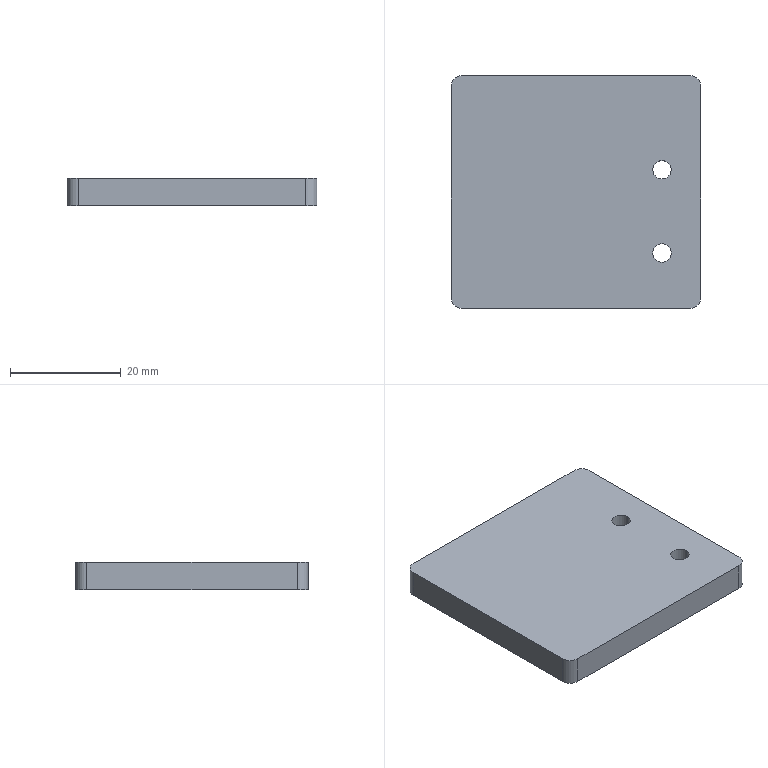Part | STEP file | H_ND24021-JJ-05-02C-BJ | 1 solid | 14 faces | box 45 x 42 x 5 mm | volume 9347 mm3 | cylinder 8 | plane 6 | commonest cylinder face diameters 3.3 x4 4 x4
STEP:
#1=CARTESIAN_POINT('',(0.,0.,0.));
#2=DIRECTION('',(0.,0.,1.));
#3=DIRECTION('',(1.,0.,0.));
#4=AXIS2_PLACEMENT_3D('',#1,#2,#3);
#5=CARTESIAN_POINT('',(-8.65,25.,0.));
#6=VERTEX_POINT('',#5);
#7=CARTESIAN_POINT('',(-8.65,25.,-5.));
#8=VERTEX_POINT('',#7);
#9=CARTESIAN_POINT('',(-8.65,25.,-5.));
#10=DIRECTION('',(0.,0.,-1.));
#11=VECTOR('',#10,1.);
#12=LINE('',#9,#11);
#13=CARTESIAN_POINT('',(-7.,25.,-5.));
#14=DIRECTION('',(0.,0.,-1.));
#15=DIRECTION('',(-1.,0.,0.));
#16=AXIS2_PLACEMENT_3D('',#13,#14,#15);
#17=CYLINDRICAL_SURFACE('',#16,1.65);
#18=CARTESIAN_POINT('',(6.283,0.));
#19=DIRECTION('',(0.,1.));
#20=VECTOR('',#19,1.);
#21=LINE('',#18,#20);
#22=(GEOMETRIC_REPRESENTATION_CONTEXT(2)PARAMETRIC_REPRESENTATION_CONTEXT()REPRESENTATION_CONTEXT('',''));
#23=DEFINITIONAL_REPRESENTATION('',(#21),#22);
#24=PCURVE('',#17,#23);
#25=CARTESIAN_POINT('',(-7.,25.,-5.));
#26=DIRECTION('',(0.,0.,-1.));
#27=DIRECTION('',(-1.,0.,0.));
#28=AXIS2_PLACEMENT_3D('',#25,#26,#27);
#29=CYLINDRICAL_SURFACE('',#28,1.65);
#30=CARTESIAN_POINT('',(0.,0.));
#31=DIRECTION('',(0.,1.));
#32=VECTOR('',#31,1.);
#33=LINE('',#30,#32);
#34=(GEOMETRIC_REPRESENTATION_CONTEXT(2)PARAMETRIC_REPRESENTATION_CONTEXT()REPRESENTATION_CONTEXT('',''));
#35=DEFINITIONAL_REPRESENTATION('',(#33),#34);
#36=PCURVE('',#29,#35);
#37=SURFACE_CURVE('',#12,(#24,#36),.PCURVE_S1.);
#38=EDGE_CURVE('',#6,#8,#37,.T.);
#39=ORIENTED_EDGE('',*,*,#38,.T.);
#40=CARTESIAN_POINT('',(-5.35,25.,-5.));
#41=VERTEX_POINT('',#40);
#42=CARTESIAN_POINT('',(-7.,25.,-5.));
#43=DIRECTION('',(0.,0.,-1.));
#44=DIRECTION('',(-1.,0.,0.));
#45=AXIS2_PLACEMENT_3D('',#42,#43,#44);
#46=CIRCLE('',#45,1.65);
#47=CARTESIAN_POINT('',(0.,0.));
#48=DIRECTION('',(1.,0.));
#49=VECTOR('',#48,1.);
#50=LINE('',#47,#49);
#51=(GEOMETRIC_REPRESENTATION_CONTEXT(2)PARAMETRIC_REPRESENTATION_CONTEXT()REPRESENTATION_CONTEXT('',''));
#52=DEFINITIONAL_REPRESENTATION('',(#50),#51);
#53=PCURVE('',#17,#52);
#54=CARTESIAN_POINT('',(0.,0.,-5.));
#55=DIRECTION('',(0.,0.,1.));
#56=DIRECTION('',(1.,0.,0.));
#57=AXIS2_PLACEMENT_3D('',#54,#55,#56);
#58=PLANE('',#57);
#59=CARTESIAN_POINT('',(-8.65,25.));
#60=CARTESIAN_POINT('',(-8.65,27.858));
#61=CARTESIAN_POINT('',(-6.175,26.429));
#62=CARTESIAN_POINT('',(-3.7,25.));
#63=CARTESIAN_POINT('',(-6.175,23.571));
#64=CARTESIAN_POINT('',(-8.65,22.142));
#65=CARTESIAN_POINT('',(-8.65,25.));
#66=(BOUNDED_CURVE()B_SPLINE_CURVE(2,(#59,#60,#61,#62,#63,#64,#65),.UNSPECIFIED.,.T.,.F.)B_SPLINE_CURVE_WITH_KNOTS((1,2,2,2,2,1),(-2.094,0.,2.094,4.189,6.283,8.378),.UNSPECIFIED.)CURVE()GEOMETRIC_REPRESENTATION_ITEM()RATIONAL_B_SPLINE_CURVE((1.,0.5,1.,0.5,1.,0.5,1.))REPRESENTATION_ITEM(''));
#67=(GEOMETRIC_REPRESENTATION_CONTEXT(2)PARAMETRIC_REPRESENTATION_CONTEXT()REPRESENTATION_CONTEXT('',''));
#68=DEFINITIONAL_REPRESENTATION('',(#66),#67);
#69=PCURVE('',#58,#68);
#70=SURFACE_CURVE('',#46,(#53,#69),.PCURVE_S1.);
#71=EDGE_CURVE('',#41,#8,#70,.T.);
#72=ORIENTED_EDGE('',*,*,#71,.F.);
#73=CARTESIAN_POINT('',(-5.35,25.,0.));
#74=VERTEX_POINT('',#73);
#75=CARTESIAN_POINT('',(-5.35,25.,-5.));
#76=DIRECTION('',(0.,0.,-1.));
#77=VECTOR('',#76,1.);
#78=LINE('',#75,#77);
#79=CARTESIAN_POINT('',(3.142,0.));
#80=DIRECTION('',(0.,1.));
#81=VECTOR('',#80,1.);
#82=LINE('',#79,#81);
#83=(GEOMETRIC_REPRESENTATION_CONTEXT(2)PARAMETRIC_REPRESENTATION_CONTEXT()REPRESENTATION_CONTEXT('',''));
#84=DEFINITIONAL_REPRESENTATION('',(#82),#83);
#85=PCURVE('',#17,#84);
#86=CARTESIAN_POINT('',(3.142,0.));
#87=DIRECTION('',(0.,1.));
#88=VECTOR('',#87,1.);
#89=LINE('',#86,#88);
#90=(GEOMETRIC_REPRESENTATION_CONTEXT(2)PARAMETRIC_REPRESENTATION_CONTEXT()REPRESENTATION_CONTEXT('',''));
#91=DEFINITIONAL_REPRESENTATION('',(#89),#90);
#92=PCURVE('',#29,#91);
#93=SURFACE_CURVE('',#78,(#85,#92),.PCURVE_S1.);
#94=EDGE_CURVE('',#74,#41,#93,.T.);
#95=ORIENTED_EDGE('',*,*,#94,.F.);
#96=CARTESIAN_POINT('',(-7.,25.,0.));
#97=DIRECTION('',(0.,0.,-1.));
#98=DIRECTION('',(-1.,0.,0.));
#99=AXIS2_PLACEMENT_3D('',#96,#97,#98);
#100=CIRCLE('',#99,1.65);
#101=CARTESIAN_POINT('',(0.,-5.));
#102=DIRECTION('',(1.,0.));
#103=VECTOR('',#102,1.);
#104=LINE('',#101,#103);
#105=(GEOMETRIC_REPRESENTATION_CONTEXT(2)PARAMETRIC_REPRESENTATION_CONTEXT()REPRESENTATION_CONTEXT('',''));
#106=DEFINITIONAL_REPRESENTATION('',(#104),#105);
#107=PCURVE('',#17,#106);
#108=CARTESIAN_POINT('',(0.,0.,0.));
#109=DIRECTION('',(0.,0.,1.));
#110=DIRECTION('',(1.,0.,0.));
#111=AXIS2_PLACEMENT_3D('',#108,#109,#110);
#112=PLANE('',#111);
#113=CARTESIAN_POINT('',(-8.65,25.));
#114=CARTESIAN_POINT('',(-8.65,27.858));
#115=CARTESIAN_POINT('',(-6.175,26.429));
#116=CARTESIAN_POINT('',(-3.7,25.));
#117=CARTESIAN_POINT('',(-6.175,23.571));
#118=CARTESIAN_POINT('',(-8.65,22.142));
#119=CARTESIAN_POINT('',(-8.65,25.));
#120=(BOUNDED_CURVE()B_SPLINE_CURVE(2,(#113,#114,#115,#116,#117,#118,#119),.UNSPECIFIED.,.T.,.F.)B_SPLINE_CURVE_WITH_KNOTS((1,2,2,2,2,1),(-2.094,0.,2.094,4.189,6.283,8.378),.UNSPECIFIED.)CURVE()GEOMETRIC_REPRESENTATION_ITEM()RATIONAL_B_SPLINE_CURVE((1.,0.5,1.,0.5,1.,0.5,1.))REPRESENTATION_ITEM(''));
#121=(GEOMETRIC_REPRESENTATION_CONTEXT(2)PARAMETRIC_REPRESENTATION_CONTEXT()REPRESENTATION_CONTEXT('',''));
#122=DEFINITIONAL_REPRESENTATION('',(#120),#121);
#123=PCURVE('',#112,#122);
#124=SURFACE_CURVE('',#100,(#107,#123),.PCURVE_S1.);
#125=EDGE_CURVE('',#74,#6,#124,.T.);
#126=ORIENTED_EDGE('',*,*,#125,.T.);
#127=EDGE_LOOP('',(#39,#72,#95,#126));
#128=FACE_BOUND('',#127,.F.);
#129=ADVANCED_FACE('',(#128),#17,.F.);
#130=CARTESIAN_POINT('',(-8.65,10.,0.));
#131=VERTEX_POINT('',#130);
#132=CARTESIAN_POINT('',(-8.65,10.,-5.));
#133=VERTEX_POINT('',#132);
#134=CARTESIAN_POINT('',(-8.65,10.,-5.));
#135=DIRECTION('',(0.,0.,-1.));
#136=VECTOR('',#135,1.);
#137=LINE('',#134,#136);
#138=CARTESIAN_POINT('',(-7.,10.,-5.));
#139=DIRECTION('',(0.,0.,-1.));
#140=DIRECTION('',(-1.,0.,0.));
#141=AXIS2_PLACEMENT_3D('',#138,#139,#140);
#142=CYLINDRICAL_SURFACE('',#141,1.65);
#143=CARTESIAN_POINT('',(6.283,0.));
#144=DIRECTION('',(0.,1.));
#145=VECTOR('',#144,1.);
#146=LINE('',#143,#145);
#147=(GEOMETRIC_REPRESENTATION_CONTEXT(2)PARAMETRIC_REPRESENTATION_CONTEXT()REPRESENTATION_CONTEXT('',''));
#148=DEFINITIONAL_REPRESENTATION('',(#146),#147);
#149=PCURVE('',#142,#148);
#150=CARTESIAN_POINT('',(-7.,10.,-5.));
#151=DIRECTION('',(0.,0.,-1.));
#152=DIRECTION('',(-1.,0.,0.));
#153=AXIS2_PLACEMENT_3D('',#150,#151,#152);
#154=CYLINDRICAL_SURFACE('',#153,1.65);
#155=CARTESIAN_POINT('',(0.,0.));
#156=DIRECTION('',(0.,1.));
#157=VECTOR('',#156,1.);
#158=LINE('',#155,#157);
#159=(GEOMETRIC_REPRESENTATION_CONTEXT(2)PARAMETRIC_REPRESENTATION_CONTEXT()REPRESENTATION_CONTEXT('',''));
#160=DEFINITIONAL_REPRESENTATION('',(#158),#159);
#161=PCURVE('',#154,#160);
#162=SURFACE_CURVE('',#137,(#149,#161),.PCURVE_S1.);
#163=EDGE_CURVE('',#131,#133,#162,.T.);
#164=ORIENTED_EDGE('',*,*,#163,.T.);
#165=CARTESIAN_POINT('',(-5.35,10.,-5.));
#166=VERTEX_POINT('',#165);
#167=CARTESIAN_POINT('',(-7.,10.,-5.));
#168=DIRECTION('',(0.,0.,-1.));
#169=DIRECTION('',(-1.,0.,0.));
#170=AXIS2_PLACEMENT_3D('',#167,#168,#169);
#171=CIRCLE('',#170,1.65);
#172=CARTESIAN_POINT('',(0.,0.));
#173=DIRECTION('',(1.,0.));
#174=VECTOR('',#173,1.);
#175=LINE('',#172,#174);
#176=(GEOMETRIC_REPRESENTATION_CONTEXT(2)PARAMETRIC_REPRESENTATION_CONTEXT()REPRESENTATION_CONTEXT('',''));
#177=DEFINITIONAL_REPRESENTATION('',(#175),#176);
#178=PCURVE('',#142,#177);
#179=CARTESIAN_POINT('',(-8.65,10.));
#180=CARTESIAN_POINT('',(-8.65,12.858));
#181=CARTESIAN_POINT('',(-6.175,11.429));
#182=CARTESIAN_POINT('',(-3.7,10.));
#183=CARTESIAN_POINT('',(-6.175,8.571));
#184=CARTESIAN_POINT('',(-8.65,7.142));
#185=CARTESIAN_POINT('',(-8.65,10.));
#186=(BOUNDED_CURVE()B_SPLINE_CURVE(2,(#179,#180,#181,#182,#183,#184,#185),.UNSPECIFIED.,.T.,.F.)B_SPLINE_CURVE_WITH_KNOTS((1,2,2,2,2,1),(-2.094,0.,2.094,4.189,6.283,8.378),.UNSPECIFIED.)CURVE()GEOMETRIC_REPRESENTATION_ITEM()RATIONAL_B_SPLINE_CURVE((1.,0.5,1.,0.5,1.,0.5,1.))REPRESENTATION_ITEM(''));
#187=(GEOMETRIC_REPRESENTATION_CONTEXT(2)PARAMETRIC_REPRESENTATION_CONTEXT()REPRESENTATION_CONTEXT('',''));
#188=DEFINITIONAL_REPRESENTATION('',(#186),#187);
#189=PCURVE('',#58,#188);
#190=SURFACE_CURVE('',#171,(#178,#189),.PCURVE_S1.);
#191=EDGE_CURVE('',#166,#133,#190,.T.);
#192=ORIENTED_EDGE('',*,*,#191,.F.);
#193=CARTESIAN_POINT('',(-5.35,10.,0.));
#194=VERTEX_POINT('',#193);
#195=CARTESIAN_POINT('',(-5.35,10.,-5.));
#196=DIRECTION('',(0.,0.,-1.));
#197=VECTOR('',#196,1.);
#198=LINE('',#195,#197);
#199=CARTESIAN_POINT('',(3.142,0.));
#200=DIRECTION('',(0.,1.));
#201=VECTOR('',#200,1.);
#202=LINE('',#199,#201);
#203=(GEOMETRIC_REPRESENTATION_CONTEXT(2)PARAMETRIC_REPRESENTATION_CONTEXT()REPRESENTATION_CONTEXT('',''));
#204=DEFINITIONAL_REPRESENTATION('',(#202),#203);
#205=PCURVE('',#142,#204);
#206=CARTESIAN_POINT('',(3.142,0.));
#207=DIRECTION('',(0.,1.));
#208=VECTOR('',#207,1.);
#209=LINE('',#206,#208);
#210=(GEOMETRIC_REPRESENTATION_CONTEXT(2)PARAMETRIC_REPRESENTATION_CONTEXT()REPRESENTATION_CONTEXT('',''));
#211=DEFINITIONAL_REPRESENTATION('',(#209),#210);
#212=PCURVE('',#154,#211);
#213=SURFACE_CURVE('',#198,(#205,#212),.PCURVE_S1.);
#214=EDGE_CURVE('',#194,#166,#213,.T.);
#215=ORIENTED_EDGE('',*,*,#214,.F.);
#216=CARTESIAN_POINT('',(-7.,10.,0.));
#217=DIRECTION('',(0.,0.,-1.));
#218=DIRECTION('',(-1.,0.,0.));
#219=AXIS2_PLACEMENT_3D('',#216,#217,#218);
#220=CIRCLE('',#219,1.65);
#221=CARTESIAN_POINT('',(0.,-5.));
#222=DIRECTION('',(1.,0.));
#223=VECTOR('',#222,1.);
#224=LINE('',#221,#223);
#225=(GEOMETRIC_REPRESENTATION_CONTEXT(2)PARAMETRIC_REPRESENTATION_CONTEXT()REPRESENTATION_CONTEXT('',''));
#226=DEFINITIONAL_REPRESENTATION('',(#224),#225);
#227=PCURVE('',#142,#226);
#228=CARTESIAN_POINT('',(-8.65,10.));
#229=CARTESIAN_POINT('',(-8.65,12.858));
#230=CARTESIAN_POINT('',(-6.175,11.429));
#231=CARTESIAN_POINT('',(-3.7,10.));
#232=CARTESIAN_POINT('',(-6.175,8.571));
#233=CARTESIAN_POINT('',(-8.65,7.142));
#234=CARTESIAN_POINT('',(-8.65,10.));
#235=(BOUNDED_CURVE()B_SPLINE_CURVE(2,(#228,#229,#230,#231,#232,#233,#234),.UNSPECIFIED.,.T.,.F.)B_SPLINE_CURVE_WITH_KNOTS((1,2,2,2,2,1),(-2.094,0.,2.094,4.189,6.283,8.378),.UNSPECIFIED.)CURVE()GEOMETRIC_REPRESENTATION_ITEM()RATIONAL_B_SPLINE_CURVE((1.,0.5,1.,0.5,1.,0.5,1.))REPRESENTATION_ITEM(''));
#236=(GEOMETRIC_REPRESENTATION_CONTEXT(2)PARAMETRIC_REPRESENTATION_CONTEXT()REPRESENTATION_CONTEXT('',''));
#237=DEFINITIONAL_REPRESENTATION('',(#235),#236);
#238=PCURVE('',#112,#237);
#239=SURFACE_CURVE('',#220,(#227,#238),.PCURVE_S1.);
#240=EDGE_CURVE('',#194,#131,#239,.T.);
#241=ORIENTED_EDGE('',*,*,#240,.T.);
#242=EDGE_LOOP('',(#164,#192,#215,#241));
#243=FACE_BOUND('',#242,.F.);
#244=ADVANCED_FACE('',(#243),#142,.F.);
#245=CARTESIAN_POINT('',(0.,2.,0.));
#246=VERTEX_POINT('',#245);
#247=CARTESIAN_POINT('',(0.,40.,0.));
#248=VERTEX_POINT('',#247);
#249=CARTESIAN_POINT('',(0.,0.,0.));
#250=DIRECTION('',(0.,1.,0.));
#251=VECTOR('',#250,1.);
#252=LINE('',#249,#251);
#253=CARTESIAN_POINT('',(0.,0.,-5.));
#254=DIRECTION('',(1.,0.,0.));
#255=DIRECTION('',(0.,1.,0.));
#256=AXIS2_PLACEMENT_3D('',#253,#254,#255);
#257=PLANE('',#256);
#258=CARTESIAN_POINT('',(0.,5.));
#259=DIRECTION('',(1.,0.));
#260=VECTOR('',#259,1.);
#261=LINE('',#258,#260);
#262=(GEOMETRIC_REPRESENTATION_CONTEXT(2)PARAMETRIC_REPRESENTATION_CONTEXT()REPRESENTATION_CONTEXT('',''));
#263=DEFINITIONAL_REPRESENTATION('',(#261),#262);
#264=PCURVE('',#257,#263);
#265=CARTESIAN_POINT('',(0.,0.));
#266=DIRECTION('',(0.,1.));
#267=VECTOR('',#266,1.);
#268=LINE('',#265,#267);
#269=(GEOMETRIC_REPRESENTATION_CONTEXT(2)PARAMETRIC_REPRESENTATION_CONTEXT()REPRESENTATION_CONTEXT('',''));
#270=DEFINITIONAL_REPRESENTATION('',(#268),#269);
#271=PCURVE('',#112,#270);
#272=SURFACE_CURVE('',#252,(#264,#271),.PCURVE_S1.);
#273=EDGE_CURVE('',#246,#248,#272,.T.);
#274=ORIENTED_EDGE('',*,*,#273,.F.);
#275=CARTESIAN_POINT('',(0.,2.,-5.));
#276=VERTEX_POINT('',#275);
#277=CARTESIAN_POINT('',(0.,2.,-5.));
#278=DIRECTION('',(0.,0.,-1.));
#279=VECTOR('',#278,1.);
#280=LINE('',#277,#279);
#281=CARTESIAN_POINT('',(2.,0.));
#282=DIRECTION('',(0.,-1.));
#283=VECTOR('',#282,1.);
#284=LINE('',#281,#283);
#285=(GEOMETRIC_REPRESENTATION_CONTEXT(2)PARAMETRIC_REPRESENTATION_CONTEXT()REPRESENTATION_CONTEXT('',''));
#286=DEFINITIONAL_REPRESENTATION('',(#284),#285);
#287=PCURVE('',#257,#286);
#288=CARTESIAN_POINT('',(-2.,2.,-5.));
#289=DIRECTION('',(0.,0.,1.));
#290=DIRECTION('',(1.,0.,0.));
#291=AXIS2_PLACEMENT_3D('',#288,#289,#290);
#292=CYLINDRICAL_SURFACE('',#291,2.);
#293=CARTESIAN_POINT('',(6.283,0.));
#294=DIRECTION('',(0.,-1.));
#295=VECTOR('',#294,1.);
#296=LINE('',#293,#295);
#297=(GEOMETRIC_REPRESENTATION_CONTEXT(2)PARAMETRIC_REPRESENTATION_CONTEXT()REPRESENTATION_CONTEXT('',''));
#298=DEFINITIONAL_REPRESENTATION('',(#296),#297);
#299=PCURVE('',#292,#298);
#300=SURFACE_CURVE('',#280,(#287,#299),.PCURVE_S1.);
#301=EDGE_CURVE('',#246,#276,#300,.T.);
#302=ORIENTED_EDGE('',*,*,#301,.T.);
#303=CARTESIAN_POINT('',(0.,40.,-5.));
#304=VERTEX_POINT('',#303);
#305=CARTESIAN_POINT('',(0.,0.,-5.));
#306=DIRECTION('',(0.,1.,0.));
#307=VECTOR('',#306,1.);
#308=LINE('',#305,#307);
#309=CARTESIAN_POINT('',(0.,0.));
#310=DIRECTION('',(1.,0.));
#311=VECTOR('',#310,1.);
#312=LINE('',#309,#311);
#313=(GEOMETRIC_REPRESENTATION_CONTEXT(2)PARAMETRIC_REPRESENTATION_CONTEXT()REPRESENTATION_CONTEXT('',''));
#314=DEFINITIONAL_REPRESENTATION('',(#312),#313);
#315=PCURVE('',#257,#314);
#316=CARTESIAN_POINT('',(0.,0.));
#317=DIRECTION('',(0.,1.));
#318=VECTOR('',#317,1.);
#319=LINE('',#316,#318);
#320=(GEOMETRIC_REPRESENTATION_CONTEXT(2)PARAMETRIC_REPRESENTATION_CONTEXT()REPRESENTATION_CONTEXT('',''));
#321=DEFINITIONAL_REPRESENTATION('',(#319),#320);
#322=PCURVE('',#58,#321);
#323=SURFACE_CURVE('',#308,(#315,#322),.PCURVE_S1.);
#324=EDGE_CURVE('',#276,#304,#323,.T.);
#325=ORIENTED_EDGE('',*,*,#324,.T.);
#326=CARTESIAN_POINT('',(0.,40.,-5.));
#327=DIRECTION('',(0.,0.,1.));
#328=VECTOR('',#327,1.);
#329=LINE('',#326,#328);
#330=CARTESIAN_POINT('',(40.,0.));
#331=DIRECTION('',(0.,1.));
#332=VECTOR('',#331,1.);
#333=LINE('',#330,#332);
#334=(GEOMETRIC_REPRESENTATION_CONTEXT(2)PARAMETRIC_REPRESENTATION_CONTEXT()REPRESENTATION_CONTEXT('',''));
#335=DEFINITIONAL_REPRESENTATION('',(#333),#334);
#336=PCURVE('',#257,#335);
#337=CARTESIAN_POINT('',(-2.,40.,-5.));
#338=DIRECTION('',(0.,0.,1.));
#339=DIRECTION('',(1.,0.,0.));
#340=AXIS2_PLACEMENT_3D('',#337,#338,#339);
#341=CYLINDRICAL_SURFACE('',#340,2.);
#342=CARTESIAN_POINT('',(0.,0.));
#343=DIRECTION('',(0.,1.));
#344=VECTOR('',#343,1.);
#345=LINE('',#342,#344);
#346=(GEOMETRIC_REPRESENTATION_CONTEXT(2)PARAMETRIC_REPRESENTATION_CONTEXT()REPRESENTATION_CONTEXT('',''));
#347=DEFINITIONAL_REPRESENTATION('',(#345),#346);
#348=PCURVE('',#341,#347);
#349=SURFACE_CURVE('',#329,(#336,#348),.PCURVE_S1.);
#350=EDGE_CURVE('',#304,#248,#349,.T.);
#351=ORIENTED_EDGE('',*,*,#350,.T.);
#352=EDGE_LOOP('',(#274,#302,#325,#351));
#353=FACE_BOUND('',#352,.T.);
#354=ADVANCED_FACE('',(#353),#257,.T.);
#355=CARTESIAN_POINT('',(-43.,0.,0.));
#356=VERTEX_POINT('',#355);
#357=CARTESIAN_POINT('',(-2.,0.,0.));
#358=VERTEX_POINT('',#357);
#359=CARTESIAN_POINT('',(0.,0.,0.));
#360=DIRECTION('',(1.,0.,0.));
#361=VECTOR('',#360,1.);
#362=LINE('',#359,#361);
#363=CARTESIAN_POINT('',(0.,0.,-5.));
#364=DIRECTION('',(0.,-1.,0.));
#365=DIRECTION('',(1.,0.,0.));
#366=AXIS2_PLACEMENT_3D('',#363,#364,#365);
#367=PLANE('',#366);
#368=CARTESIAN_POINT('',(0.,5.));
#369=DIRECTION('',(1.,0.));
#370=VECTOR('',#369,1.);
#371=LINE('',#368,#370);
#372=(GEOMETRIC_REPRESENTATION_CONTEXT(2)PARAMETRIC_REPRESENTATION_CONTEXT()REPRESENTATION_CONTEXT('',''));
#373=DEFINITIONAL_REPRESENTATION('',(#371),#372);
#374=PCURVE('',#367,#373);
#375=CARTESIAN_POINT('',(0.,0.));
#376=DIRECTION('',(1.,0.));
#377=VECTOR('',#376,1.);
#378=LINE('',#375,#377);
#379=(GEOMETRIC_REPRESENTATION_CONTEXT(2)PARAMETRIC_REPRESENTATION_CONTEXT()REPRESENTATION_CONTEXT('',''));
#380=DEFINITIONAL_REPRESENTATION('',(#378),#379);
#381=PCURVE('',#112,#380);
#382=SURFACE_CURVE('',#362,(#374,#381),.PCURVE_S1.);
#383=EDGE_CURVE('',#356,#358,#382,.T.);
#384=ORIENTED_EDGE('',*,*,#383,.F.);
#385=CARTESIAN_POINT('',(-43.,0.,-5.));
#386=VERTEX_POINT('',#385);
#387=CARTESIAN_POINT('',(-43.,0.,-5.));
#388=DIRECTION('',(0.,0.,-1.));
#389=VECTOR('',#388,1.);
#390=LINE('',#387,#389);
#391=CARTESIAN_POINT('',(-43.,0.));
#392=DIRECTION('',(0.,-1.));
#393=VECTOR('',#392,1.);
#394=LINE('',#391,#393);
#395=(GEOMETRIC_REPRESENTATION_CONTEXT(2)PARAMETRIC_REPRESENTATION_CONTEXT()REPRESENTATION_CONTEXT('',''));
#396=DEFINITIONAL_REPRESENTATION('',(#394),#395);
#397=PCURVE('',#367,#396);
#398=CARTESIAN_POINT('',(-43.,2.,-5.));
#399=DIRECTION('',(0.,0.,1.));
#400=DIRECTION('',(1.,0.,0.));
#401=AXIS2_PLACEMENT_3D('',#398,#399,#400);
#402=CYLINDRICAL_SURFACE('',#401,2.);
#403=CARTESIAN_POINT('',(4.712,0.));
#404=DIRECTION('',(0.,-1.));
#405=VECTOR('',#404,1.);
#406=LINE('',#403,#405);
#407=(GEOMETRIC_REPRESENTATION_CONTEXT(2)PARAMETRIC_REPRESENTATION_CONTEXT()REPRESENTATION_CONTEXT('',''));
#408=DEFINITIONAL_REPRESENTATION('',(#406),#407);
#409=PCURVE('',#402,#408);
#410=SURFACE_CURVE('',#390,(#397,#409),.PCURVE_S1.);
#411=EDGE_CURVE('',#356,#386,#410,.T.);
#412=ORIENTED_EDGE('',*,*,#411,.T.);
#413=CARTESIAN_POINT('',(-2.,0.,-5.));
#414=VERTEX_POINT('',#413);
#415=CARTESIAN_POINT('',(0.,0.,-5.));
#416=DIRECTION('',(1.,0.,0.));
#417=VECTOR('',#416,1.);
#418=LINE('',#415,#417);
#419=CARTESIAN_POINT('',(0.,0.));
#420=DIRECTION('',(1.,0.));
#421=VECTOR('',#420,1.);
#422=LINE('',#419,#421);
#423=(GEOMETRIC_REPRESENTATION_CONTEXT(2)PARAMETRIC_REPRESENTATION_CONTEXT()REPRESENTATION_CONTEXT('',''));
#424=DEFINITIONAL_REPRESENTATION('',(#422),#423);
#425=PCURVE('',#367,#424);
#426=CARTESIAN_POINT('',(0.,0.));
#427=DIRECTION('',(1.,0.));
#428=VECTOR('',#427,1.);
#429=LINE('',#426,#428);
#430=(GEOMETRIC_REPRESENTATION_CONTEXT(2)PARAMETRIC_REPRESENTATION_CONTEXT()REPRESENTATION_CONTEXT('',''));
#431=DEFINITIONAL_REPRESENTATION('',(#429),#430);
#432=PCURVE('',#58,#431);
#433=SURFACE_CURVE('',#418,(#425,#432),.PCURVE_S1.);
#434=EDGE_CURVE('',#386,#414,#433,.T.);
#435=ORIENTED_EDGE('',*,*,#434,.T.);
#436=CARTESIAN_POINT('',(-2.,0.,-5.));
#437=DIRECTION('',(0.,0.,1.));
#438=VECTOR('',#437,1.);
#439=LINE('',#436,#438);
#440=CARTESIAN_POINT('',(-2.,0.));
#441=DIRECTION('',(0.,1.));
#442=VECTOR('',#441,1.);
#443=LINE('',#440,#442);
#444=(GEOMETRIC_REPRESENTATION_CONTEXT(2)PARAMETRIC_REPRESENTATION_CONTEXT()REPRESENTATION_CONTEXT('',''));
#445=DEFINITIONAL_REPRESENTATION('',(#443),#444);
#446=PCURVE('',#367,#445);
#447=CARTESIAN_POINT('',(4.712,0.));
#448=DIRECTION('',(0.,1.));
#449=VECTOR('',#448,1.);
#450=LINE('',#447,#449);
#451=(GEOMETRIC_REPRESENTATION_CONTEXT(2)PARAMETRIC_REPRESENTATION_CONTEXT()REPRESENTATION_CONTEXT('',''));
#452=DEFINITIONAL_REPRESENTATION('',(#450),#451);
#453=PCURVE('',#292,#452);
#454=SURFACE_CURVE('',#439,(#446,#453),.PCURVE_S1.);
#455=EDGE_CURVE('',#414,#358,#454,.T.);
#456=ORIENTED_EDGE('',*,*,#455,.T.);
#457=EDGE_LOOP('',(#384,#412,#435,#456));
#458=FACE_BOUND('',#457,.T.);
#459=ADVANCED_FACE('',(#458),#367,.T.);
#460=CARTESIAN_POINT('',(-45.,40.,-5.));
#461=VERTEX_POINT('',#460);
#462=CARTESIAN_POINT('',(-45.,2.,-5.));
#463=VERTEX_POINT('',#462);
#464=CARTESIAN_POINT('',(-45.,0.,-5.));
#465=DIRECTION('',(0.,-1.,0.));
#466=VECTOR('',#465,1.);
#467=LINE('',#464,#466);
#468=CARTESIAN_POINT('',(-45.,0.,-5.));
#469=DIRECTION('',(-1.,0.,0.));
#470=DIRECTION('',(0.,0.,1.));
#471=AXIS2_PLACEMENT_3D('',#468,#469,#470);
#472=PLANE('',#471);
#473=CARTESIAN_POINT('',(0.,0.));
#474=DIRECTION('',(0.,-1.));
#475=VECTOR('',#474,1.);
#476=LINE('',#473,#475);
#477=(GEOMETRIC_REPRESENTATION_CONTEXT(2)PARAMETRIC_REPRESENTATION_CONTEXT()REPRESENTATION_CONTEXT('',''));
#478=DEFINITIONAL_REPRESENTATION('',(#476),#477);
#479=PCURVE('',#472,#478);
#480=CARTESIAN_POINT('',(-45.,0.));
#481=DIRECTION('',(0.,-1.));
#482=VECTOR('',#481,1.);
#483=LINE('',#480,#482);
#484=(GEOMETRIC_REPRESENTATION_CONTEXT(2)PARAMETRIC_REPRESENTATION_CONTEXT()REPRESENTATION_CONTEXT('',''));
#485=DEFINITIONAL_REPRESENTATION('',(#483),#484);
#486=PCURVE('',#58,#485);
#487=SURFACE_CURVE('',#467,(#479,#486),.PCURVE_S1.);
#488=EDGE_CURVE('',#461,#463,#487,.T.);
#489=ORIENTED_EDGE('',*,*,#488,.T.);
#490=CARTESIAN_POINT('',(-45.,2.,0.));
#491=VERTEX_POINT('',#490);
#492=CARTESIAN_POINT('',(-45.,2.,-5.));
#493=DIRECTION('',(0.,0.,1.));
#494=VECTOR('',#493,1.);
#495=LINE('',#492,#494);
#496=CARTESIAN_POINT('',(0.,2.));
#497=DIRECTION('',(1.,0.));
#498=VECTOR('',#497,1.);
#499=LINE('',#496,#498);
#500=(GEOMETRIC_REPRESENTATION_CONTEXT(2)PARAMETRIC_REPRESENTATION_CONTEXT()REPRESENTATION_CONTEXT('',''));
#501=DEFINITIONAL_REPRESENTATION('',(#499),#500);
#502=PCURVE('',#472,#501);
#503=CARTESIAN_POINT('',(3.142,0.));
#504=DIRECTION('',(0.,1.));
#505=VECTOR('',#504,1.);
#506=LINE('',#503,#505);
#507=(GEOMETRIC_REPRESENTATION_CONTEXT(2)PARAMETRIC_REPRESENTATION_CONTEXT()REPRESENTATION_CONTEXT('',''));
#508=DEFINITIONAL_REPRESENTATION('',(#506),#507);
#509=PCURVE('',#402,#508);
#510=SURFACE_CURVE('',#495,(#502,#509),.PCURVE_S1.);
#511=EDGE_CURVE('',#463,#491,#510,.T.);
#512=ORIENTED_EDGE('',*,*,#511,.T.);
#513=CARTESIAN_POINT('',(-45.,40.,0.));
#514=VERTEX_POINT('',#513);
#515=CARTESIAN_POINT('',(-45.,0.,0.));
#516=DIRECTION('',(0.,-1.,0.));
#517=VECTOR('',#516,1.);
#518=LINE('',#515,#517);
#519=CARTESIAN_POINT('',(5.,0.));
#520=DIRECTION('',(0.,-1.));
#521=VECTOR('',#520,1.);
#522=LINE('',#519,#521);
#523=(GEOMETRIC_REPRESENTATION_CONTEXT(2)PARAMETRIC_REPRESENTATION_CONTEXT()REPRESENTATION_CONTEXT('',''));
#524=DEFINITIONAL_REPRESENTATION('',(#522),#523);
#525=PCURVE('',#472,#524);
#526=CARTESIAN_POINT('',(-45.,0.));
#527=DIRECTION('',(0.,-1.));
#528=VECTOR('',#527,1.);
#529=LINE('',#526,#528);
#530=(GEOMETRIC_REPRESENTATION_CONTEXT(2)PARAMETRIC_REPRESENTATION_CONTEXT()REPRESENTATION_CONTEXT('',''));
#531=DEFINITIONAL_REPRESENTATION('',(#529),#530);
#532=PCURVE('',#112,#531);
#533=SURFACE_CURVE('',#518,(#525,#532),.PCURVE_S1.);
#534=EDGE_CURVE('',#514,#491,#533,.T.);
#535=ORIENTED_EDGE('',*,*,#534,.F.);
#536=CARTESIAN_POINT('',(-45.,40.,-5.));
#537=DIRECTION('',(0.,0.,-1.));
#538=VECTOR('',#537,1.);
#539=LINE('',#536,#538);
#540=CARTESIAN_POINT('',(0.,40.));
#541=DIRECTION('',(-1.,0.));
#542=VECTOR('',#541,1.);
#543=LINE('',#540,#542);
#544=(GEOMETRIC_REPRESENTATION_CONTEXT(2)PARAMETRIC_REPRESENTATION_CONTEXT()REPRESENTATION_CONTEXT('',''));
#545=DEFINITIONAL_REPRESENTATION('',(#543),#544);
#546=PCURVE('',#472,#545);
#547=CARTESIAN_POINT('',(-43.,40.,-5.));
#548=DIRECTION('',(0.,0.,1.));
#549=DIRECTION('',(1.,0.,0.));
#550=AXIS2_PLACEMENT_3D('',#547,#548,#549);
#551=CYLINDRICAL_SURFACE('',#550,2.);
#552=CARTESIAN_POINT('',(3.142,0.));
#553=DIRECTION('',(0.,-1.));
#554=VECTOR('',#553,1.);
#555=LINE('',#552,#554);
#556=(GEOMETRIC_REPRESENTATION_CONTEXT(2)PARAMETRIC_REPRESENTATION_CONTEXT()REPRESENTATION_CONTEXT('',''));
#557=DEFINITIONAL_REPRESENTATION('',(#555),#556);
#558=PCURVE('',#551,#557);
#559=SURFACE_CURVE('',#539,(#546,#558),.PCURVE_S1.);
#560=EDGE_CURVE('',#514,#461,#559,.T.);
#561=ORIENTED_EDGE('',*,*,#560,.T.);
#562=EDGE_LOOP('',(#489,#512,#535,#561));
#563=FACE_BOUND('',#562,.T.);
#564=ADVANCED_FACE('',(#563),#472,.T.);
#565=CARTESIAN_POINT('',(-2.,42.,-5.));
#566=VERTEX_POINT('',#565);
#567=CARTESIAN_POINT('',(-43.,42.,-5.));
#568=VERTEX_POINT('',#567);
#569=CARTESIAN_POINT('',(0.,42.,-5.));
#570=DIRECTION('',(-1.,0.,0.));
#571=VECTOR('',#570,1.);
#572=LINE('',#569,#571);
#573=CARTESIAN_POINT('',(0.,42.,-5.));
#574=DIRECTION('',(0.,1.,0.));
#575=DIRECTION('',(-1.,0.,0.));
#576=AXIS2_PLACEMENT_3D('',#573,#574,#575);
#577=PLANE('',#576);
#578=CARTESIAN_POINT('',(0.,0.));
#579=DIRECTION('',(1.,0.));
#580=VECTOR('',#579,1.);
#581=LINE('',#578,#580);
#582=(GEOMETRIC_REPRESENTATION_CONTEXT(2)PARAMETRIC_REPRESENTATION_CONTEXT()REPRESENTATION_CONTEXT('',''));
#583=DEFINITIONAL_REPRESENTATION('',(#581),#582);
#584=PCURVE('',#577,#583);
#585=CARTESIAN_POINT('',(0.,42.));
#586=DIRECTION('',(-1.,0.));
#587=VECTOR('',#586,1.);
#588=LINE('',#585,#587);
#589=(GEOMETRIC_REPRESENTATION_CONTEXT(2)PARAMETRIC_REPRESENTATION_CONTEXT()REPRESENTATION_CONTEXT('',''));
#590=DEFINITIONAL_REPRESENTATION('',(#588),#589);
#591=PCURVE('',#58,#590);
#592=SURFACE_CURVE('',#572,(#584,#591),.PCURVE_S1.);
#593=EDGE_CURVE('',#566,#568,#592,.T.);
#594=ORIENTED_EDGE('',*,*,#593,.T.);
#595=CARTESIAN_POINT('',(-43.,42.,0.));
#596=VERTEX_POINT('',#595);
#597=CARTESIAN_POINT('',(-43.,42.,-5.));
#598=DIRECTION('',(0.,0.,1.));
#599=VECTOR('',#598,1.);
#600=LINE('',#597,#599);
#601=CARTESIAN_POINT('',(43.,0.));
#602=DIRECTION('',(0.,1.));
#603=VECTOR('',#602,1.);
#604=LINE('',#601,#603);
#605=(GEOMETRIC_REPRESENTATION_CONTEXT(2)PARAMETRIC_REPRESENTATION_CONTEXT()REPRESENTATION_CONTEXT('',''));
#606=DEFINITIONAL_REPRESENTATION('',(#604),#605);
#607=PCURVE('',#577,#606);
#608=CARTESIAN_POINT('',(1.571,0.));
#609=DIRECTION('',(0.,1.));
#610=VECTOR('',#609,1.);
#611=LINE('',#608,#610);
#612=(GEOMETRIC_REPRESENTATION_CONTEXT(2)PARAMETRIC_REPRESENTATION_CONTEXT()REPRESENTATION_CONTEXT('',''));
#613=DEFINITIONAL_REPRESENTATION('',(#611),#612);
#614=PCURVE('',#551,#613);
#615=SURFACE_CURVE('',#600,(#607,#614),.PCURVE_S1.);
#616=EDGE_CURVE('',#568,#596,#615,.T.);
#617=ORIENTED_EDGE('',*,*,#616,.T.);
#618=CARTESIAN_POINT('',(-2.,42.,0.));
#619=VERTEX_POINT('',#618);
#620=CARTESIAN_POINT('',(0.,42.,0.));
#621=DIRECTION('',(-1.,0.,0.));
#622=VECTOR('',#621,1.);
#623=LINE('',#620,#622);
#624=CARTESIAN_POINT('',(0.,5.));
#625=DIRECTION('',(1.,0.));
#626=VECTOR('',#625,1.);
#627=LINE('',#624,#626);
#628=(GEOMETRIC_REPRESENTATION_CONTEXT(2)PARAMETRIC_REPRESENTATION_CONTEXT()REPRESENTATION_CONTEXT('',''));
#629=DEFINITIONAL_REPRESENTATION('',(#627),#628);
#630=PCURVE('',#577,#629);
#631=CARTESIAN_POINT('',(0.,42.));
#632=DIRECTION('',(-1.,0.));
#633=VECTOR('',#632,1.);
#634=LINE('',#631,#633);
#635=(GEOMETRIC_REPRESENTATION_CONTEXT(2)PARAMETRIC_REPRESENTATION_CONTEXT()REPRESENTATION_CONTEXT('',''));
#636=DEFINITIONAL_REPRESENTATION('',(#634),#635);
#637=PCURVE('',#112,#636);
#638=SURFACE_CURVE('',#623,(#630,#637),.PCURVE_S1.);
#639=EDGE_CURVE('',#619,#596,#638,.T.);
#640=ORIENTED_EDGE('',*,*,#639,.F.);
#641=CARTESIAN_POINT('',(-2.,42.,-5.));
#642=DIRECTION('',(0.,0.,-1.));
#643=VECTOR('',#642,1.);
#644=LINE('',#641,#643);
#645=CARTESIAN_POINT('',(2.,0.));
#646=DIRECTION('',(0.,-1.));
#647=VECTOR('',#646,1.);
#648=LINE('',#645,#647);
#649=(GEOMETRIC_REPRESENTATION_CONTEXT(2)PARAMETRIC_REPRESENTATION_CONTEXT()REPRESENTATION_CONTEXT('',''));
#650=DEFINITIONAL_REPRESENTATION('',(#648),#649);
#651=PCURVE('',#577,#650);
#652=CARTESIAN_POINT('',(1.571,0.));
#653=DIRECTION('',(0.,-1.));
#654=VECTOR('',#653,1.);
#655=LINE('',#652,#654);
#656=(GEOMETRIC_REPRESENTATION_CONTEXT(2)PARAMETRIC_REPRESENTATION_CONTEXT()REPRESENTATION_CONTEXT('',''));
#657=DEFINITIONAL_REPRESENTATION('',(#655),#656);
#658=PCURVE('',#341,#657);
#659=SURFACE_CURVE('',#644,(#651,#658),.PCURVE_S1.);
#660=EDGE_CURVE('',#619,#566,#659,.T.);
#661=ORIENTED_EDGE('',*,*,#660,.T.);
#662=EDGE_LOOP('',(#594,#617,#640,#661));
#663=FACE_BOUND('',#662,.T.);
#664=ADVANCED_FACE('',(#663),#577,.T.);
#665=CARTESIAN_POINT('',(-7.,25.,-5.));
#666=DIRECTION('',(0.,0.,-1.));
#667=DIRECTION('',(-1.,0.,0.));
#668=AXIS2_PLACEMENT_3D('',#665,#666,#667);
#669=CIRCLE('',#668,1.65);
#670=CARTESIAN_POINT('',(-8.65,25.));
#671=CARTESIAN_POINT('',(-8.65,27.858));
#672=CARTESIAN_POINT('',(-6.175,26.429));
#673=CARTESIAN_POINT('',(-3.7,25.));
#674=CARTESIAN_POINT('',(-6.175,23.571));
#675=CARTESIAN_POINT('',(-8.65,22.142));
#676=CARTESIAN_POINT('',(-8.65,25.));
#677=(BOUNDED_CURVE()B_SPLINE_CURVE(2,(#670,#671,#672,#673,#674,#675,#676),.UNSPECIFIED.,.T.,.F.)B_SPLINE_CURVE_WITH_KNOTS((1,2,2,2,2,1),(-2.094,0.,2.094,4.189,6.283,8.378),.UNSPECIFIED.)CURVE()GEOMETRIC_REPRESENTATION_ITEM()RATIONAL_B_SPLINE_CURVE((1.,0.5,1.,0.5,1.,0.5,1.))REPRESENTATION_ITEM(''));
#678=(GEOMETRIC_REPRESENTATION_CONTEXT(2)PARAMETRIC_REPRESENTATION_CONTEXT()REPRESENTATION_CONTEXT('',''));
#679=DEFINITIONAL_REPRESENTATION('',(#677),#678);
#680=PCURVE('',#58,#679);
#681=CARTESIAN_POINT('',(0.,0.));
#682=DIRECTION('',(1.,0.));
#683=VECTOR('',#682,1.);
#684=LINE('',#681,#683);
#685=(GEOMETRIC_REPRESENTATION_CONTEXT(2)PARAMETRIC_REPRESENTATION_CONTEXT()REPRESENTATION_CONTEXT('',''));
#686=DEFINITIONAL_REPRESENTATION('',(#684),#685);
#687=PCURVE('',#29,#686);
#688=SURFACE_CURVE('',#669,(#680,#687),.PCURVE_S1.);
#689=EDGE_CURVE('',#8,#41,#688,.T.);
#690=ORIENTED_EDGE('',*,*,#689,.F.);
#691=ORIENTED_EDGE('',*,*,#71,.F.);
#692=EDGE_LOOP('',(#690,#691));
#693=FACE_BOUND('',#692,.T.);
#694=CARTESIAN_POINT('',(-7.,10.,-5.));
#695=DIRECTION('',(0.,0.,-1.));
#696=DIRECTION('',(-1.,0.,0.));
#697=AXIS2_PLACEMENT_3D('',#694,#695,#696);
#698=CIRCLE('',#697,1.65);
#699=CARTESIAN_POINT('',(-8.65,10.));
#700=CARTESIAN_POINT('',(-8.65,12.858));
#701=CARTESIAN_POINT('',(-6.175,11.429));
#702=CARTESIAN_POINT('',(-3.7,10.));
#703=CARTESIAN_POINT('',(-6.175,8.571));
#704=CARTESIAN_POINT('',(-8.65,7.142));
#705=CARTESIAN_POINT('',(-8.65,10.));
#706=(BOUNDED_CURVE()B_SPLINE_CURVE(2,(#699,#700,#701,#702,#703,#704,#705),.UNSPECIFIED.,.T.,.F.)B_SPLINE_CURVE_WITH_KNOTS((1,2,2,2,2,1),(-2.094,0.,2.094,4.189,6.283,8.378),.UNSPECIFIED.)CURVE()GEOMETRIC_REPRESENTATION_ITEM()RATIONAL_B_SPLINE_CURVE((1.,0.5,1.,0.5,1.,0.5,1.))REPRESENTATION_ITEM(''));
#707=(GEOMETRIC_REPRESENTATION_CONTEXT(2)PARAMETRIC_REPRESENTATION_CONTEXT()REPRESENTATION_CONTEXT('',''));
#708=DEFINITIONAL_REPRESENTATION('',(#706),#707);
#709=PCURVE('',#58,#708);
#710=CARTESIAN_POINT('',(0.,0.));
#711=DIRECTION('',(1.,0.));
#712=VECTOR('',#711,1.);
#713=LINE('',#710,#712);
#714=(GEOMETRIC_REPRESENTATION_CONTEXT(2)PARAMETRIC_REPRESENTATION_CONTEXT()REPRESENTATION_CONTEXT('',''));
#715=DEFINITIONAL_REPRESENTATION('',(#713),#714);
#716=PCURVE('',#154,#715);
#717=SURFACE_CURVE('',#698,(#709,#716),.PCURVE_S1.);
#718=EDGE_CURVE('',#133,#166,#717,.T.);
#719=ORIENTED_EDGE('',*,*,#718,.F.);
#720=ORIENTED_EDGE('',*,*,#191,.F.);
#721=EDGE_LOOP('',(#719,#720));
#722=FACE_BOUND('',#721,.T.);
#723=ORIENTED_EDGE('',*,*,#434,.F.);
#724=CARTESIAN_POINT('',(-43.,2.,-5.));
#725=DIRECTION('',(0.,0.,-1.));
#726=DIRECTION('',(1.,0.,0.));
#727=AXIS2_PLACEMENT_3D('',#724,#725,#726);
#728=CIRCLE('',#727,2.);
#729=CARTESIAN_POINT('',(-41.,2.));
#730=CARTESIAN_POINT('',(-41.,-1.464));
#731=CARTESIAN_POINT('',(-44.,0.2679));
#732=CARTESIAN_POINT('',(-47.,2.));
#733=CARTESIAN_POINT('',(-44.,3.732));
#734=CARTESIAN_POINT('',(-41.,5.464));
#735=CARTESIAN_POINT('',(-41.,2.));
#736=(BOUNDED_CURVE()B_SPLINE_CURVE(2,(#729,#730,#731,#732,#733,#734,#735),.UNSPECIFIED.,.T.,.F.)B_SPLINE_CURVE_WITH_KNOTS((1,2,2,2,2,1),(-2.094,0.,2.094,4.189,6.283,8.378),.UNSPECIFIED.)CURVE()GEOMETRIC_REPRESENTATION_ITEM()RATIONAL_B_SPLINE_CURVE((1.,0.5,1.,0.5,1.,0.5,1.))REPRESENTATION_ITEM(''));
#737=(GEOMETRIC_REPRESENTATION_CONTEXT(2)PARAMETRIC_REPRESENTATION_CONTEXT()REPRESENTATION_CONTEXT('',''));
#738=DEFINITIONAL_REPRESENTATION('',(#736),#737);
#739=PCURVE('',#58,#738);
#740=CARTESIAN_POINT('',(6.283,0.));
#741=DIRECTION('',(-1.,0.));
#742=VECTOR('',#741,1.);
#743=LINE('',#740,#742);
#744=(GEOMETRIC_REPRESENTATION_CONTEXT(2)PARAMETRIC_REPRESENTATION_CONTEXT()REPRESENTATION_CONTEXT('',''));
#745=DEFINITIONAL_REPRESENTATION('',(#743),#744);
#746=PCURVE('',#402,#745);
#747=SURFACE_CURVE('',#728,(#739,#746),.PCURVE_S1.);
#748=EDGE_CURVE('',#386,#463,#747,.T.);
#749=ORIENTED_EDGE('',*,*,#748,.T.);
#750=ORIENTED_EDGE('',*,*,#488,.F.);
#751=CARTESIAN_POINT('',(-43.,40.,-5.));
#752=DIRECTION('',(0.,0.,-1.));
#753=DIRECTION('',(1.,0.,0.));
#754=AXIS2_PLACEMENT_3D('',#751,#752,#753);
#755=CIRCLE('',#754,2.);
#756=CARTESIAN_POINT('',(-41.,40.));
#757=CARTESIAN_POINT('',(-41.,36.536));
#758=CARTESIAN_POINT('',(-44.,38.268));
#759=CARTESIAN_POINT('',(-47.,40.));
#760=CARTESIAN_POINT('',(-44.,41.732));
#761=CARTESIAN_POINT('',(-41.,43.464));
#762=CARTESIAN_POINT('',(-41.,40.));
#763=(BOUNDED_CURVE()B_SPLINE_CURVE(2,(#756,#757,#758,#759,#760,#761,#762),.UNSPECIFIED.,.T.,.F.)B_SPLINE_CURVE_WITH_KNOTS((1,2,2,2,2,1),(-2.094,0.,2.094,4.189,6.283,8.378),.UNSPECIFIED.)CURVE()GEOMETRIC_REPRESENTATION_ITEM()RATIONAL_B_SPLINE_CURVE((1.,0.5,1.,0.5,1.,0.5,1.))REPRESENTATION_ITEM(''));
#764=(GEOMETRIC_REPRESENTATION_CONTEXT(2)PARAMETRIC_REPRESENTATION_CONTEXT()REPRESENTATION_CONTEXT('',''));
#765=DEFINITIONAL_REPRESENTATION('',(#763),#764);
#766=PCURVE('',#58,#765);
#767=CARTESIAN_POINT('',(6.283,0.));
#768=DIRECTION('',(-1.,0.));
#769=VECTOR('',#768,1.);
#770=LINE('',#767,#769);
#771=(GEOMETRIC_REPRESENTATION_CONTEXT(2)PARAMETRIC_REPRESENTATION_CONTEXT()REPRESENTATION_CONTEXT('',''));
#772=DEFINITIONAL_REPRESENTATION('',(#770),#771);
#773=PCURVE('',#551,#772);
#774=SURFACE_CURVE('',#755,(#766,#773),.PCURVE_S1.);
#775=EDGE_CURVE('',#461,#568,#774,.T.);
#776=ORIENTED_EDGE('',*,*,#775,.T.);
#777=ORIENTED_EDGE('',*,*,#593,.F.);
#778=CARTESIAN_POINT('',(-2.,40.,-5.));
#779=DIRECTION('',(0.,0.,-1.));
#780=DIRECTION('',(1.,0.,0.));
#781=AXIS2_PLACEMENT_3D('',#778,#779,#780);
#782=CIRCLE('',#781,2.);
#783=CARTESIAN_POINT('',(0.,40.));
#784=CARTESIAN_POINT('',(0.,36.536));
#785=CARTESIAN_POINT('',(-3.,38.268));
#786=CARTESIAN_POINT('',(-6.,40.));
#787=CARTESIAN_POINT('',(-3.,41.732));
#788=CARTESIAN_POINT('',(0.,43.464));
#789=CARTESIAN_POINT('',(0.,40.));
#790=(BOUNDED_CURVE()B_SPLINE_CURVE(2,(#783,#784,#785,#786,#787,#788,#789),.UNSPECIFIED.,.T.,.F.)B_SPLINE_CURVE_WITH_KNOTS((1,2,2,2,2,1),(-2.094,0.,2.094,4.189,6.283,8.378),.UNSPECIFIED.)CURVE()GEOMETRIC_REPRESENTATION_ITEM()RATIONAL_B_SPLINE_CURVE((1.,0.5,1.,0.5,1.,0.5,1.))REPRESENTATION_ITEM(''));
#791=(GEOMETRIC_REPRESENTATION_CONTEXT(2)PARAMETRIC_REPRESENTATION_CONTEXT()REPRESENTATION_CONTEXT('',''));
#792=DEFINITIONAL_REPRESENTATION('',(#790),#791);
#793=PCURVE('',#58,#792);
#794=CARTESIAN_POINT('',(6.283,0.));
#795=DIRECTION('',(-1.,0.));
#796=VECTOR('',#795,1.);
#797=LINE('',#794,#796);
#798=(GEOMETRIC_REPRESENTATION_CONTEXT(2)PARAMETRIC_REPRESENTATION_CONTEXT()REPRESENTATION_CONTEXT('',''));
#799=DEFINITIONAL_REPRESENTATION('',(#797),#798);
#800=PCURVE('',#341,#799);
#801=SURFACE_CURVE('',#782,(#793,#800),.PCURVE_S1.);
#802=EDGE_CURVE('',#566,#304,#801,.T.);
#803=ORIENTED_EDGE('',*,*,#802,.T.);
#804=ORIENTED_EDGE('',*,*,#324,.F.);
#805=CARTESIAN_POINT('',(-2.,2.,-5.));
#806=DIRECTION('',(0.,0.,-1.));
#807=DIRECTION('',(1.,0.,0.));
#808=AXIS2_PLACEMENT_3D('',#805,#806,#807);
#809=CIRCLE('',#808,2.);
#810=CARTESIAN_POINT('',(0.,2.));
#811=CARTESIAN_POINT('',(0.,-1.464));
#812=CARTESIAN_POINT('',(-3.,0.2679));
#813=CARTESIAN_POINT('',(-6.,2.));
#814=CARTESIAN_POINT('',(-3.,3.732));
#815=CARTESIAN_POINT('',(0.,5.464));
#816=CARTESIAN_POINT('',(0.,2.));
#817=(BOUNDED_CURVE()B_SPLINE_CURVE(2,(#810,#811,#812,#813,#814,#815,#816),.UNSPECIFIED.,.T.,.F.)B_SPLINE_CURVE_WITH_KNOTS((1,2,2,2,2,1),(-2.094,0.,2.094,4.189,6.283,8.378),.UNSPECIFIED.)CURVE()GEOMETRIC_REPRESENTATION_ITEM()RATIONAL_B_SPLINE_CURVE((1.,0.5,1.,0.5,1.,0.5,1.))REPRESENTATION_ITEM(''));
#818=(GEOMETRIC_REPRESENTATION_CONTEXT(2)PARAMETRIC_REPRESENTATION_CONTEXT()REPRESENTATION_CONTEXT('',''));
#819=DEFINITIONAL_REPRESENTATION('',(#817),#818);
#820=PCURVE('',#58,#819);
#821=CARTESIAN_POINT('',(6.283,0.));
#822=DIRECTION('',(-1.,0.));
#823=VECTOR('',#822,1.);
#824=LINE('',#821,#823);
#825=(GEOMETRIC_REPRESENTATION_CONTEXT(2)PARAMETRIC_REPRESENTATION_CONTEXT()REPRESENTATION_CONTEXT('',''));
#826=DEFINITIONAL_REPRESENTATION('',(#824),#825);
#827=PCURVE('',#292,#826);
#828=SURFACE_CURVE('',#809,(#820,#827),.PCURVE_S1.);
#829=EDGE_CURVE('',#276,#414,#828,.T.);
#830=ORIENTED_EDGE('',*,*,#829,.T.);
#831=EDGE_LOOP('',(#723,#749,#750,#776,#777,#803,#804,#830));
#832=FACE_BOUND('',#831,.T.);
#833=ADVANCED_FACE('',(#693,#722,#832),#58,.F.);
#834=CARTESIAN_POINT('',(-7.,25.,0.));
#835=DIRECTION('',(0.,0.,-1.));
#836=DIRECTION('',(-1.,0.,0.));
#837=AXIS2_PLACEMENT_3D('',#834,#835,#836);
#838=CIRCLE('',#837,1.65);
#839=CARTESIAN_POINT('',(-8.65,25.));
#840=CARTESIAN_POINT('',(-8.65,27.858));
#841=CARTESIAN_POINT('',(-6.175,26.429));
#842=CARTESIAN_POINT('',(-3.7,25.));
#843=CARTESIAN_POINT('',(-6.175,23.571));
#844=CARTESIAN_POINT('',(-8.65,22.142));
#845=CARTESIAN_POINT('',(-8.65,25.));
#846=(BOUNDED_CURVE()B_SPLINE_CURVE(2,(#839,#840,#841,#842,#843,#844,#845),.UNSPECIFIED.,.T.,.F.)B_SPLINE_CURVE_WITH_KNOTS((1,2,2,2,2,1),(-2.094,0.,2.094,4.189,6.283,8.378),.UNSPECIFIED.)CURVE()GEOMETRIC_REPRESENTATION_ITEM()RATIONAL_B_SPLINE_CURVE((1.,0.5,1.,0.5,1.,0.5,1.))REPRESENTATION_ITEM(''));
#847=(GEOMETRIC_REPRESENTATION_CONTEXT(2)PARAMETRIC_REPRESENTATION_CONTEXT()REPRESENTATION_CONTEXT('',''));
#848=DEFINITIONAL_REPRESENTATION('',(#846),#847);
#849=PCURVE('',#112,#848);
#850=CARTESIAN_POINT('',(0.,-5.));
#851=DIRECTION('',(1.,0.));
#852=VECTOR('',#851,1.);
#853=LINE('',#850,#852);
#854=(GEOMETRIC_REPRESENTATION_CONTEXT(2)PARAMETRIC_REPRESENTATION_CONTEXT()REPRESENTATION_CONTEXT('',''));
#855=DEFINITIONAL_REPRESENTATION('',(#853),#854);
#856=PCURVE('',#29,#855);
#857=SURFACE_CURVE('',#838,(#849,#856),.PCURVE_S1.);
#858=EDGE_CURVE('',#6,#74,#857,.T.);
#859=ORIENTED_EDGE('',*,*,#858,.T.);
#860=ORIENTED_EDGE('',*,*,#125,.T.);
#861=EDGE_LOOP('',(#859,#860));
#862=FACE_BOUND('',#861,.T.);
#863=CARTESIAN_POINT('',(-7.,10.,0.));
#864=DIRECTION('',(0.,0.,-1.));
#865=DIRECTION('',(-1.,0.,0.));
#866=AXIS2_PLACEMENT_3D('',#863,#864,#865);
#867=CIRCLE('',#866,1.65);
#868=CARTESIAN_POINT('',(-8.65,10.));
#869=CARTESIAN_POINT('',(-8.65,12.858));
#870=CARTESIAN_POINT('',(-6.175,11.429));
#871=CARTESIAN_POINT('',(-3.7,10.));
#872=CARTESIAN_POINT('',(-6.175,8.571));
#873=CARTESIAN_POINT('',(-8.65,7.142));
#874=CARTESIAN_POINT('',(-8.65,10.));
#875=(BOUNDED_CURVE()B_SPLINE_CURVE(2,(#868,#869,#870,#871,#872,#873,#874),.UNSPECIFIED.,.T.,.F.)B_SPLINE_CURVE_WITH_KNOTS((1,2,2,2,2,1),(-2.094,0.,2.094,4.189,6.283,8.378),.UNSPECIFIED.)CURVE()GEOMETRIC_REPRESENTATION_ITEM()RATIONAL_B_SPLINE_CURVE((1.,0.5,1.,0.5,1.,0.5,1.))REPRESENTATION_ITEM(''));
#876=(GEOMETRIC_REPRESENTATION_CONTEXT(2)PARAMETRIC_REPRESENTATION_CONTEXT()REPRESENTATION_CONTEXT('',''));
#877=DEFINITIONAL_REPRESENTATION('',(#875),#876);
#878=PCURVE('',#112,#877);
#879=CARTESIAN_POINT('',(0.,-5.));
#880=DIRECTION('',(1.,0.));
#881=VECTOR('',#880,1.);
#882=LINE('',#879,#881);
#883=(GEOMETRIC_REPRESENTATION_CONTEXT(2)PARAMETRIC_REPRESENTATION_CONTEXT()REPRESENTATION_CONTEXT('',''));
#884=DEFINITIONAL_REPRESENTATION('',(#882),#883);
#885=PCURVE('',#154,#884);
#886=SURFACE_CURVE('',#867,(#878,#885),.PCURVE_S1.);
#887=EDGE_CURVE('',#131,#194,#886,.T.);
#888=ORIENTED_EDGE('',*,*,#887,.T.);
#889=ORIENTED_EDGE('',*,*,#240,.T.);
#890=EDGE_LOOP('',(#888,#889));
#891=FACE_BOUND('',#890,.T.);
#892=ORIENTED_EDGE('',*,*,#534,.T.);
#893=CARTESIAN_POINT('',(-43.,2.,0.));
#894=DIRECTION('',(0.,0.,1.));
#895=DIRECTION('',(1.,0.,0.));
#896=AXIS2_PLACEMENT_3D('',#893,#894,#895);
#897=CIRCLE('',#896,2.);
#898=CARTESIAN_POINT('',(-43.,2.));
#899=DIRECTION('',(1.,0.));
#900=AXIS2_PLACEMENT_2D('',#898,#899);
#901=CIRCLE('',#900,2.);
#902=(GEOMETRIC_REPRESENTATION_CONTEXT(2)PARAMETRIC_REPRESENTATION_CONTEXT()REPRESENTATION_CONTEXT('',''));
#903=DEFINITIONAL_REPRESENTATION('',(#901),#902);
#904=PCURVE('',#112,#903);
#905=CARTESIAN_POINT('',(0.,5.));
#906=DIRECTION('',(1.,0.));
#907=VECTOR('',#906,1.);
#908=LINE('',#905,#907);
#909=(GEOMETRIC_REPRESENTATION_CONTEXT(2)PARAMETRIC_REPRESENTATION_CONTEXT()REPRESENTATION_CONTEXT('',''));
#910=DEFINITIONAL_REPRESENTATION('',(#908),#909);
#911=PCURVE('',#402,#910);
#912=SURFACE_CURVE('',#897,(#904,#911),.PCURVE_S1.);
#913=EDGE_CURVE('',#491,#356,#912,.T.);
#914=ORIENTED_EDGE('',*,*,#913,.T.);
#915=ORIENTED_EDGE('',*,*,#383,.T.);
#916=CARTESIAN_POINT('',(-2.,2.,0.));
#917=DIRECTION('',(0.,0.,1.));
#918=DIRECTION('',(1.,0.,0.));
#919=AXIS2_PLACEMENT_3D('',#916,#917,#918);
#920=CIRCLE('',#919,2.);
#921=CARTESIAN_POINT('',(-2.,2.));
#922=DIRECTION('',(1.,0.));
#923=AXIS2_PLACEMENT_2D('',#921,#922);
#924=CIRCLE('',#923,2.);
#925=(GEOMETRIC_REPRESENTATION_CONTEXT(2)PARAMETRIC_REPRESENTATION_CONTEXT()REPRESENTATION_CONTEXT('',''));
#926=DEFINITIONAL_REPRESENTATION('',(#924),#925);
#927=PCURVE('',#112,#926);
#928=CARTESIAN_POINT('',(0.,5.));
#929=DIRECTION('',(1.,0.));
#930=VECTOR('',#929,1.);
#931=LINE('',#928,#930);
#932=(GEOMETRIC_REPRESENTATION_CONTEXT(2)PARAMETRIC_REPRESENTATION_CONTEXT()REPRESENTATION_CONTEXT('',''));
#933=DEFINITIONAL_REPRESENTATION('',(#931),#932);
#934=PCURVE('',#292,#933);
#935=SURFACE_CURVE('',#920,(#927,#934),.PCURVE_S1.);
#936=EDGE_CURVE('',#358,#246,#935,.T.);
#937=ORIENTED_EDGE('',*,*,#936,.T.);
#938=ORIENTED_EDGE('',*,*,#273,.T.);
#939=CARTESIAN_POINT('',(-2.,40.,0.));
#940=DIRECTION('',(0.,0.,1.));
#941=DIRECTION('',(1.,0.,0.));
#942=AXIS2_PLACEMENT_3D('',#939,#940,#941);
#943=CIRCLE('',#942,2.);
#944=CARTESIAN_POINT('',(-2.,40.));
#945=DIRECTION('',(1.,0.));
#946=AXIS2_PLACEMENT_2D('',#944,#945);
#947=CIRCLE('',#946,2.);
#948=(GEOMETRIC_REPRESENTATION_CONTEXT(2)PARAMETRIC_REPRESENTATION_CONTEXT()REPRESENTATION_CONTEXT('',''));
#949=DEFINITIONAL_REPRESENTATION('',(#947),#948);
#950=PCURVE('',#112,#949);
#951=CARTESIAN_POINT('',(0.,5.));
#952=DIRECTION('',(1.,0.));
#953=VECTOR('',#952,1.);
#954=LINE('',#951,#953);
#955=(GEOMETRIC_REPRESENTATION_CONTEXT(2)PARAMETRIC_REPRESENTATION_CONTEXT()REPRESENTATION_CONTEXT('',''));
#956=DEFINITIONAL_REPRESENTATION('',(#954),#955);
#957=PCURVE('',#341,#956);
#958=SURFACE_CURVE('',#943,(#950,#957),.PCURVE_S1.);
#959=EDGE_CURVE('',#248,#619,#958,.T.);
#960=ORIENTED_EDGE('',*,*,#959,.T.);
#961=ORIENTED_EDGE('',*,*,#639,.T.);
#962=CARTESIAN_POINT('',(-43.,40.,0.));
#963=DIRECTION('',(0.,0.,1.));
#964=DIRECTION('',(1.,0.,0.));
#965=AXIS2_PLACEMENT_3D('',#962,#963,#964);
#966=CIRCLE('',#965,2.);
#967=CARTESIAN_POINT('',(-43.,40.));
#968=DIRECTION('',(1.,0.));
#969=AXIS2_PLACEMENT_2D('',#967,#968);
#970=CIRCLE('',#969,2.);
#971=(GEOMETRIC_REPRESENTATION_CONTEXT(2)PARAMETRIC_REPRESENTATION_CONTEXT()REPRESENTATION_CONTEXT('',''));
#972=DEFINITIONAL_REPRESENTATION('',(#970),#971);
#973=PCURVE('',#112,#972);
#974=CARTESIAN_POINT('',(0.,5.));
#975=DIRECTION('',(1.,0.));
#976=VECTOR('',#975,1.);
#977=LINE('',#974,#976);
#978=(GEOMETRIC_REPRESENTATION_CONTEXT(2)PARAMETRIC_REPRESENTATION_CONTEXT()REPRESENTATION_CONTEXT('',''));
#979=DEFINITIONAL_REPRESENTATION('',(#977),#978);
#980=PCURVE('',#551,#979);
#981=SURFACE_CURVE('',#966,(#973,#980),.PCURVE_S1.);
#982=EDGE_CURVE('',#596,#514,#981,.T.);
#983=ORIENTED_EDGE('',*,*,#982,.T.);
#984=EDGE_LOOP('',(#892,#914,#915,#937,#938,#960,#961,#983));
#985=FACE_BOUND('',#984,.T.);
#986=ADVANCED_FACE('',(#862,#891,#985),#112,.T.);
#987=ORIENTED_EDGE('',*,*,#748,.F.);
#988=ORIENTED_EDGE('',*,*,#411,.F.);
#989=ORIENTED_EDGE('',*,*,#913,.F.);
#990=ORIENTED_EDGE('',*,*,#511,.F.);
#991=EDGE_LOOP('',(#987,#988,#989,#990));
#992=FACE_BOUND('',#991,.T.);
#993=ADVANCED_FACE('',(#992),#402,.T.);
#994=ORIENTED_EDGE('',*,*,#775,.F.);
#995=ORIENTED_EDGE('',*,*,#560,.F.);
#996=ORIENTED_EDGE('',*,*,#982,.F.);
#997=ORIENTED_EDGE('',*,*,#616,.F.);
#998=EDGE_LOOP('',(#994,#995,#996,#997));
#999=FACE_BOUND('',#998,.T.);
#1000=ADVANCED_FACE('',(#999),#551,.T.);
#1001=ORIENTED_EDGE('',*,*,#829,.F.);
#1002=ORIENTED_EDGE('',*,*,#301,.F.);
#1003=ORIENTED_EDGE('',*,*,#936,.F.);
#1004=ORIENTED_EDGE('',*,*,#455,.F.);
#1005=EDGE_LOOP('',(#1001,#1002,#1003,#1004));
#1006=FACE_BOUND('',#1005,.T.);
#1007=ADVANCED_FACE('',(#1006),#292,.T.);
#1008=ORIENTED_EDGE('',*,*,#802,.F.);
#1009=ORIENTED_EDGE('',*,*,#660,.F.);
#1010=ORIENTED_EDGE('',*,*,#959,.F.);
#1011=ORIENTED_EDGE('',*,*,#350,.F.);
#1012=EDGE_LOOP('',(#1008,#1009,#1010,#1011));
#1013=FACE_BOUND('',#1012,.T.);
#1014=ADVANCED_FACE('',(#1013),#341,.T.);
#1015=ORIENTED_EDGE('',*,*,#718,.F.);
#1016=ORIENTED_EDGE('',*,*,#163,.F.);
#1017=ORIENTED_EDGE('',*,*,#887,.T.);
#1018=ORIENTED_EDGE('',*,*,#214,.T.);
#1019=EDGE_LOOP('',(#1015,#1016,#1017,#1018));
#1020=FACE_BOUND('',#1019,.F.);
#1021=ADVANCED_FACE('',(#1020),#154,.F.);
#1022=ORIENTED_EDGE('',*,*,#689,.F.);
#1023=ORIENTED_EDGE('',*,*,#38,.F.);
#1024=ORIENTED_EDGE('',*,*,#858,.T.);
#1025=ORIENTED_EDGE('',*,*,#94,.T.);
#1026=EDGE_LOOP('',(#1022,#1023,#1024,#1025));
#1027=FACE_BOUND('',#1026,.F.);
#1028=ADVANCED_FACE('',(#1027),#29,.F.);
#1029=CLOSED_SHELL('',(#129,#244,#354,#459,#564,#664,#833,#986,#993,#1000,#1007,#1014,#1021,#1028));
#1030=MANIFOLD_SOLID_BREP('',#1029);
#1031=(LENGTH_UNIT()NAMED_UNIT(*)SI_UNIT(.MILLI.,.METRE.));
#1032=UNCERTAINTY_MEASURE_WITH_UNIT(LENGTH_MEASURE(0.0000001),#1031,'','');
#1033=(NAMED_UNIT(*)PLANE_ANGLE_UNIT()SI_UNIT($,.RADIAN.));
#1034=(NAMED_UNIT(*)SI_UNIT($,.STERADIAN.)SOLID_ANGLE_UNIT());
#1035=(GEOMETRIC_REPRESENTATION_CONTEXT(3)GLOBAL_UNCERTAINTY_ASSIGNED_CONTEXT((#1032))GLOBAL_UNIT_ASSIGNED_CONTEXT((#1031,#1033,#1034))REPRESENTATION_CONTEXT('',''));
#1036=ADVANCED_BREP_SHAPE_REPRESENTATION('',(#4,#1030),#1035);